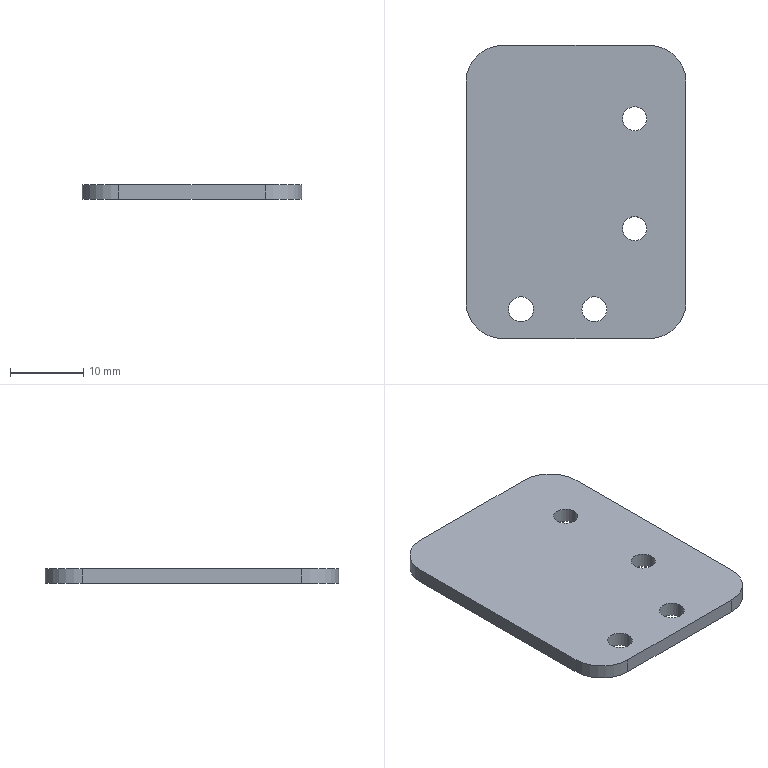Part | STEP file | H_ND24021-JJ-05-02-BJ | 1 solid | 18 faces | box 30 x 40 x 2 mm | volume 2287 mm3 | cylinder 12 | plane 6 | commonest cylinder face diameters 3.3 x4 3.4 x4 10 x4